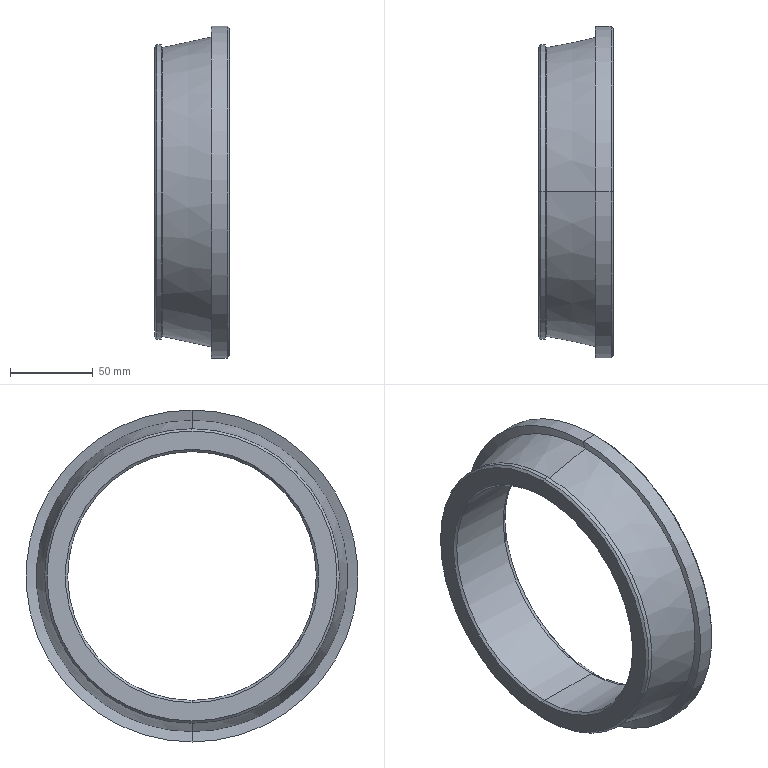Part | SolidWorks | features BaseBody 1 | 1 solid | 22 faces | box 45 x 200.13 x 200.13 mm | volume 409638 mm3 | cone 12 | cylinder 6 | plane 2 | torus 2 | commonest cylinder face diameters 150 x2 177.45 x2 200.13 x2
STEP:
#1=CARTESIAN_POINT('',(4.,0.,-76.333));
#2=VERTEX_POINT('',#1);
#3=CARTESIAN_POINT('',(4.,0.,76.333));
#4=VERTEX_POINT('',#3);
#5=CARTESIAN_POINT('',(4.,0.,0.));
#6=DIRECTION('',(1.,0.,0.));
#7=DIRECTION('',(0.,0.,-1.));
#8=AXIS2_PLACEMENT_3D('',#5,#6,#7);
#9=CIRCLE('',#8,76.333);
#10=EDGE_CURVE('',#2,#4,#9,.T.);
#11=ORIENTED_EDGE('',*,*,#10,.T.);
#12=CARTESIAN_POINT('',(4.,0.,0.));
#13=DIRECTION('',(1.,0.,0.));
#14=DIRECTION('',(0.,0.,-1.));
#15=AXIS2_PLACEMENT_3D('',#12,#13,#14);
#16=CIRCLE('',#15,76.333);
#17=EDGE_CURVE('',#4,#2,#16,.T.);
#18=ORIENTED_EDGE('',*,*,#17,.T.);
#19=EDGE_LOOP('',(#11,#18));
#20=FACE_BOUND('',#19,.T.);
#21=CARTESIAN_POINT('',(4.,0.,87.392));
#22=VERTEX_POINT('',#21);
#23=CARTESIAN_POINT('',(4.,0.,-87.392));
#24=VERTEX_POINT('',#23);
#25=CARTESIAN_POINT('',(4.,0.,0.));
#26=DIRECTION('',(1.,0.,0.));
#27=DIRECTION('',(0.,0.,-1.));
#28=AXIS2_PLACEMENT_3D('',#25,#26,#27);
#29=CIRCLE('',#28,87.392);
#30=EDGE_CURVE('',#22,#24,#29,.T.);
#31=ORIENTED_EDGE('',*,*,#30,.F.);
#32=CARTESIAN_POINT('',(4.,0.,0.));
#33=DIRECTION('',(1.,0.,0.));
#34=DIRECTION('',(0.,0.,-1.));
#35=AXIS2_PLACEMENT_3D('',#32,#33,#34);
#36=CIRCLE('',#35,87.392);
#37=EDGE_CURVE('',#24,#22,#36,.T.);
#38=ORIENTED_EDGE('',*,*,#37,.F.);
#39=EDGE_LOOP('',(#31,#38));
#40=FACE_OUTER_BOUND('',#39,.T.);
#41=CARTESIAN_POINT('',(4.,87.392,0.));
#42=DIRECTION('',(-1.,0.,0.));
#43=DIRECTION('',(0.,0.,1.));
#44=AXIS2_PLACEMENT_3D('',#41,#42,#43);
#45=PLANE('',#44);
#46=ADVANCED_FACE('',(#20,#40),#45,.T.);
#47=CARTESIAN_POINT('',(5.333,0.,88.725));
#48=VERTEX_POINT('',#47);
#49=CARTESIAN_POINT('',(4.,0.,87.392));
#50=DIRECTION('',(0.7071,0.,0.7071));
#51=VECTOR('',#50,1000.);
#52=LINE('',#49,#51);
#53=EDGE_CURVE('',#22,#48,#52,.T.);
#54=ORIENTED_EDGE('',*,*,#53,.T.);
#55=CARTESIAN_POINT('',(5.333,0.,-88.725));
#56=VERTEX_POINT('',#55);
#57=CARTESIAN_POINT('',(5.333,0.,0.));
#58=DIRECTION('',(1.,0.,0.));
#59=DIRECTION('',(0.,0.,-1.));
#60=AXIS2_PLACEMENT_3D('',#57,#58,#59);
#61=CIRCLE('',#60,88.725);
#62=EDGE_CURVE('',#56,#48,#61,.T.);
#63=ORIENTED_EDGE('',*,*,#62,.F.);
#64=CARTESIAN_POINT('',(4.,0.,-87.392));
#65=DIRECTION('',(0.7071,0.,-0.7071));
#66=VECTOR('',#65,1000.);
#67=LINE('',#64,#66);
#68=EDGE_CURVE('',#24,#56,#67,.T.);
#69=ORIENTED_EDGE('',*,*,#68,.F.);
#70=ORIENTED_EDGE('',*,*,#37,.T.);
#71=EDGE_LOOP('',(#54,#63,#69,#70));
#72=FACE_OUTER_BOUND('',#71,.T.);
#73=CARTESIAN_POINT('',(5.333,0.,0.));
#74=DIRECTION('',(1.,0.,0.));
#75=DIRECTION('',(0.,-1.,0.));
#76=AXIS2_PLACEMENT_3D('',#73,#74,#75);
#77=CONICAL_SURFACE('',#76,88.725,0.7854);
#78=ADVANCED_FACE('',(#72),#77,.T.);
#79=ORIENTED_EDGE('',*,*,#53,.F.);
#80=ORIENTED_EDGE('',*,*,#30,.T.);
#81=ORIENTED_EDGE('',*,*,#68,.T.);
#82=CARTESIAN_POINT('',(5.333,0.,0.));
#83=DIRECTION('',(1.,0.,0.));
#84=DIRECTION('',(0.,0.,-1.));
#85=AXIS2_PLACEMENT_3D('',#82,#83,#84);
#86=CIRCLE('',#85,88.725);
#87=EDGE_CURVE('',#48,#56,#86,.T.);
#88=ORIENTED_EDGE('',*,*,#87,.F.);
#89=EDGE_LOOP('',(#79,#80,#81,#88));
#90=FACE_OUTER_BOUND('',#89,.T.);
#91=CARTESIAN_POINT('',(5.333,0.,0.));
#92=DIRECTION('',(1.,0.,0.));
#93=DIRECTION('',(0.,1.,0.));
#94=AXIS2_PLACEMENT_3D('',#91,#92,#93);
#95=CONICAL_SURFACE('',#94,88.725,0.7854);
#96=ADVANCED_FACE('',(#90),#95,.T.);
#97=CARTESIAN_POINT('',(7.994,0.,88.725));
#98=VERTEX_POINT('',#97);
#99=CARTESIAN_POINT('',(5.333,0.,88.725));
#100=DIRECTION('',(1.,0.,0.));
#101=VECTOR('',#100,1000.);
#102=LINE('',#99,#101);
#103=EDGE_CURVE('',#48,#98,#102,.T.);
#104=ORIENTED_EDGE('',*,*,#103,.F.);
#105=ORIENTED_EDGE('',*,*,#87,.T.);
#106=CARTESIAN_POINT('',(7.994,0.,-88.725));
#107=VERTEX_POINT('',#106);
#108=CARTESIAN_POINT('',(5.333,0.,-88.725));
#109=DIRECTION('',(1.,0.,0.));
#110=VECTOR('',#109,1000.);
#111=LINE('',#108,#110);
#112=EDGE_CURVE('',#56,#107,#111,.T.);
#113=ORIENTED_EDGE('',*,*,#112,.T.);
#114=CARTESIAN_POINT('',(7.994,0.,0.));
#115=DIRECTION('',(1.,0.,0.));
#116=DIRECTION('',(0.,0.,-1.));
#117=AXIS2_PLACEMENT_3D('',#114,#115,#116);
#118=CIRCLE('',#117,88.725);
#119=EDGE_CURVE('',#98,#107,#118,.T.);
#120=ORIENTED_EDGE('',*,*,#119,.F.);
#121=EDGE_LOOP('',(#104,#105,#113,#120));
#122=FACE_OUTER_BOUND('',#121,.T.);
#123=CARTESIAN_POINT('',(49.,0.,0.));
#124=DIRECTION('',(1.,0.,0.));
#125=DIRECTION('',(0.,1.,0.));
#126=AXIS2_PLACEMENT_3D('',#123,#124,#125);
#127=CYLINDRICAL_SURFACE('',#126,88.725);
#128=ADVANCED_FACE('',(#122),#127,.T.);
#129=CARTESIAN_POINT('',(8.484,0.,-87.036));
#130=VERTEX_POINT('',#129);
#131=CARTESIAN_POINT('',(8.484,0.,-87.036));
#132=DIRECTION('',(-0.2785,0.,-0.9604));
#133=VECTOR('',#132,1000.);
#134=LINE('',#131,#133);
#135=EDGE_CURVE('',#130,#107,#134,.T.);
#136=ORIENTED_EDGE('',*,*,#135,.F.);
#137=CARTESIAN_POINT('',(8.484,0.,87.036));
#138=VERTEX_POINT('',#137);
#139=CARTESIAN_POINT('',(8.484,0.,0.));
#140=DIRECTION('',(1.,0.,0.));
#141=DIRECTION('',(0.,0.,-1.));
#142=AXIS2_PLACEMENT_3D('',#139,#140,#141);
#143=CIRCLE('',#142,87.036);
#144=EDGE_CURVE('',#138,#130,#143,.T.);
#145=ORIENTED_EDGE('',*,*,#144,.F.);
#146=CARTESIAN_POINT('',(8.484,0.,87.036));
#147=DIRECTION('',(-0.2785,0.,0.9604));
#148=VECTOR('',#147,1000.);
#149=LINE('',#146,#148);
#150=EDGE_CURVE('',#138,#98,#149,.T.);
#151=ORIENTED_EDGE('',*,*,#150,.T.);
#152=ORIENTED_EDGE('',*,*,#119,.T.);
#153=EDGE_LOOP('',(#136,#145,#151,#152));
#154=FACE_OUTER_BOUND('',#153,.T.);
#155=CARTESIAN_POINT('',(8.484,0.,0.));
#156=DIRECTION('',(-1.,0.,0.));
#157=DIRECTION('',(0.,1.,0.));
#158=AXIS2_PLACEMENT_3D('',#155,#156,#157);
#159=CONICAL_SURFACE('',#158,87.036,1.289);
#160=ADVANCED_FACE('',(#154),#159,.T.);
#161=ORIENTED_EDGE('',*,*,#135,.T.);
#162=CARTESIAN_POINT('',(7.994,0.,0.));
#163=DIRECTION('',(1.,0.,0.));
#164=DIRECTION('',(0.,0.,-1.));
#165=AXIS2_PLACEMENT_3D('',#162,#163,#164);
#166=CIRCLE('',#165,88.725);
#167=EDGE_CURVE('',#107,#98,#166,.T.);
#168=ORIENTED_EDGE('',*,*,#167,.T.);
#169=ORIENTED_EDGE('',*,*,#150,.F.);
#170=CARTESIAN_POINT('',(8.484,0.,0.));
#171=DIRECTION('',(1.,0.,0.));
#172=DIRECTION('',(0.,0.,-1.));
#173=AXIS2_PLACEMENT_3D('',#170,#171,#172);
#174=CIRCLE('',#173,87.036);
#175=EDGE_CURVE('',#130,#138,#174,.T.);
#176=ORIENTED_EDGE('',*,*,#175,.F.);
#177=EDGE_LOOP('',(#161,#168,#169,#176));
#178=FACE_OUTER_BOUND('',#177,.T.);
#179=CARTESIAN_POINT('',(8.484,0.,0.));
#180=DIRECTION('',(-1.,0.,0.));
#181=DIRECTION('',(0.,-1.,0.));
#182=AXIS2_PLACEMENT_3D('',#179,#180,#181);
#183=CONICAL_SURFACE('',#182,87.036,1.289);
#184=ADVANCED_FACE('',(#178),#183,.T.);
#185=CARTESIAN_POINT('',(39.843,0.,93.793));
#186=VERTEX_POINT('',#185);
#187=CARTESIAN_POINT('',(8.484,0.,87.036));
#188=DIRECTION('',(0.9776,0.,0.2107));
#189=VECTOR('',#188,1000.);
#190=LINE('',#187,#189);
#191=EDGE_CURVE('',#138,#186,#190,.T.);
#192=ORIENTED_EDGE('',*,*,#191,.T.);
#193=CARTESIAN_POINT('',(39.843,0.,-93.793));
#194=VERTEX_POINT('',#193);
#195=CARTESIAN_POINT('',(39.843,0.,0.));
#196=DIRECTION('',(1.,0.,0.));
#197=DIRECTION('',(0.,0.,-1.));
#198=AXIS2_PLACEMENT_3D('',#195,#196,#197);
#199=CIRCLE('',#198,93.793);
#200=EDGE_CURVE('',#194,#186,#199,.T.);
#201=ORIENTED_EDGE('',*,*,#200,.F.);
#202=CARTESIAN_POINT('',(8.484,0.,-87.036));
#203=DIRECTION('',(0.9776,0.,-0.2107));
#204=VECTOR('',#203,1000.);
#205=LINE('',#202,#204);
#206=EDGE_CURVE('',#130,#194,#205,.T.);
#207=ORIENTED_EDGE('',*,*,#206,.F.);
#208=ORIENTED_EDGE('',*,*,#175,.T.);
#209=EDGE_LOOP('',(#192,#201,#207,#208));
#210=FACE_OUTER_BOUND('',#209,.T.);
#211=CARTESIAN_POINT('',(39.843,0.,0.));
#212=DIRECTION('',(1.,0.,0.));
#213=DIRECTION('',(0.,-1.,0.));
#214=AXIS2_PLACEMENT_3D('',#211,#212,#213);
#215=CONICAL_SURFACE('',#214,93.793,0.2122);
#216=ADVANCED_FACE('',(#210),#215,.T.);
#217=ORIENTED_EDGE('',*,*,#191,.F.);
#218=ORIENTED_EDGE('',*,*,#144,.T.);
#219=ORIENTED_EDGE('',*,*,#206,.T.);
#220=CARTESIAN_POINT('',(39.843,0.,0.));
#221=DIRECTION('',(1.,0.,0.));
#222=DIRECTION('',(0.,0.,-1.));
#223=AXIS2_PLACEMENT_3D('',#220,#221,#222);
#224=CIRCLE('',#223,93.793);
#225=EDGE_CURVE('',#186,#194,#224,.T.);
#226=ORIENTED_EDGE('',*,*,#225,.F.);
#227=EDGE_LOOP('',(#217,#218,#219,#226));
#228=FACE_OUTER_BOUND('',#227,.T.);
#229=CARTESIAN_POINT('',(39.843,0.,0.));
#230=DIRECTION('',(1.,0.,0.));
#231=DIRECTION('',(0.,1.,0.));
#232=AXIS2_PLACEMENT_3D('',#229,#230,#231);
#233=CONICAL_SURFACE('',#232,93.793,0.2122);
#234=ADVANCED_FACE('',(#228),#233,.T.);
#235=CARTESIAN_POINT('',(38.024,0.,-100.065));
#236=VERTEX_POINT('',#235);
#237=CARTESIAN_POINT('',(39.843,0.,-93.793));
#238=DIRECTION('',(-0.2785,0.,-0.9604));
#239=VECTOR('',#238,1000.);
#240=LINE('',#237,#239);
#241=EDGE_CURVE('',#194,#236,#240,.T.);
#242=ORIENTED_EDGE('',*,*,#241,.T.);
#243=CARTESIAN_POINT('',(38.024,0.,100.065));
#244=VERTEX_POINT('',#243);
#245=CARTESIAN_POINT('',(38.024,0.,0.));
#246=DIRECTION('',(1.,0.,0.));
#247=DIRECTION('',(0.,0.,-1.));
#248=AXIS2_PLACEMENT_3D('',#245,#246,#247);
#249=CIRCLE('',#248,100.065);
#250=EDGE_CURVE('',#244,#236,#249,.T.);
#251=ORIENTED_EDGE('',*,*,#250,.F.);
#252=CARTESIAN_POINT('',(39.843,0.,93.793));
#253=DIRECTION('',(-0.2785,0.,0.9604));
#254=VECTOR('',#253,1000.);
#255=LINE('',#252,#254);
#256=EDGE_CURVE('',#186,#244,#255,.T.);
#257=ORIENTED_EDGE('',*,*,#256,.F.);
#258=ORIENTED_EDGE('',*,*,#225,.T.);
#259=EDGE_LOOP('',(#242,#251,#257,#258));
#260=FACE_OUTER_BOUND('',#259,.T.);
#261=CARTESIAN_POINT('',(38.024,0.,0.));
#262=DIRECTION('',(-1.,0.,0.));
#263=DIRECTION('',(0.,1.,0.));
#264=AXIS2_PLACEMENT_3D('',#261,#262,#263);
#265=CONICAL_SURFACE('',#264,100.065,1.289);
#266=ADVANCED_FACE('',(#260),#265,.F.);
#267=ORIENTED_EDGE('',*,*,#241,.F.);
#268=ORIENTED_EDGE('',*,*,#200,.T.);
#269=ORIENTED_EDGE('',*,*,#256,.T.);
#270=CARTESIAN_POINT('',(38.024,0.,0.));
#271=DIRECTION('',(1.,0.,0.));
#272=DIRECTION('',(0.,0.,-1.));
#273=AXIS2_PLACEMENT_3D('',#270,#271,#272);
#274=CIRCLE('',#273,100.065);
#275=EDGE_CURVE('',#236,#244,#274,.T.);
#276=ORIENTED_EDGE('',*,*,#275,.F.);
#277=EDGE_LOOP('',(#267,#268,#269,#276));
#278=FACE_OUTER_BOUND('',#277,.T.);
#279=CARTESIAN_POINT('',(38.024,0.,0.));
#280=DIRECTION('',(-1.,0.,0.));
#281=DIRECTION('',(0.,-1.,0.));
#282=AXIS2_PLACEMENT_3D('',#279,#280,#281);
#283=CONICAL_SURFACE('',#282,100.065,1.289);
#284=ADVANCED_FACE('',(#278),#283,.F.);
#285=CARTESIAN_POINT('',(47.667,0.,100.065));
#286=VERTEX_POINT('',#285);
#287=CARTESIAN_POINT('',(38.024,0.,100.065));
#288=DIRECTION('',(1.,0.,0.));
#289=VECTOR('',#288,1000.);
#290=LINE('',#287,#289);
#291=EDGE_CURVE('',#244,#286,#290,.T.);
#292=ORIENTED_EDGE('',*,*,#291,.T.);
#293=CARTESIAN_POINT('',(47.667,0.,-100.065));
#294=VERTEX_POINT('',#293);
#295=CARTESIAN_POINT('',(47.667,0.,0.));
#296=DIRECTION('',(1.,0.,0.));
#297=DIRECTION('',(0.,0.,-1.));
#298=AXIS2_PLACEMENT_3D('',#295,#296,#297);
#299=CIRCLE('',#298,100.065);
#300=EDGE_CURVE('',#294,#286,#299,.T.);
#301=ORIENTED_EDGE('',*,*,#300,.F.);
#302=CARTESIAN_POINT('',(38.024,0.,-100.065));
#303=DIRECTION('',(1.,0.,0.));
#304=VECTOR('',#303,1000.);
#305=LINE('',#302,#304);
#306=EDGE_CURVE('',#236,#294,#305,.T.);
#307=ORIENTED_EDGE('',*,*,#306,.F.);
#308=ORIENTED_EDGE('',*,*,#275,.T.);
#309=EDGE_LOOP('',(#292,#301,#307,#308));
#310=FACE_OUTER_BOUND('',#309,.T.);
#311=CARTESIAN_POINT('',(49.,0.,0.));
#312=DIRECTION('',(1.,0.,0.));
#313=DIRECTION('',(0.,-1.,0.));
#314=AXIS2_PLACEMENT_3D('',#311,#312,#313);
#315=CYLINDRICAL_SURFACE('',#314,100.065);
#316=ADVANCED_FACE('',(#310),#315,.T.);
#317=ORIENTED_EDGE('',*,*,#291,.F.);
#318=ORIENTED_EDGE('',*,*,#250,.T.);
#319=ORIENTED_EDGE('',*,*,#306,.T.);
#320=CARTESIAN_POINT('',(47.667,0.,0.));
#321=DIRECTION('',(1.,0.,0.));
#322=DIRECTION('',(0.,0.,-1.));
#323=AXIS2_PLACEMENT_3D('',#320,#321,#322);
#324=CIRCLE('',#323,100.065);
#325=EDGE_CURVE('',#286,#294,#324,.T.);
#326=ORIENTED_EDGE('',*,*,#325,.F.);
#327=EDGE_LOOP('',(#317,#318,#319,#326));
#328=FACE_OUTER_BOUND('',#327,.T.);
#329=CARTESIAN_POINT('',(49.,0.,0.));
#330=DIRECTION('',(1.,0.,0.));
#331=DIRECTION('',(0.,1.,0.));
#332=AXIS2_PLACEMENT_3D('',#329,#330,#331);
#333=CYLINDRICAL_SURFACE('',#332,100.065);
#334=ADVANCED_FACE('',(#328),#333,.T.);
#335=CARTESIAN_POINT('',(49.,0.,-98.732));
#336=VERTEX_POINT('',#335);
#337=CARTESIAN_POINT('',(49.,0.,-98.732));
#338=DIRECTION('',(-0.7071,0.,-0.7071));
#339=VECTOR('',#338,1000.);
#340=LINE('',#337,#339);
#341=EDGE_CURVE('',#336,#294,#340,.T.);
#342=ORIENTED_EDGE('',*,*,#341,.F.);
#343=CARTESIAN_POINT('',(49.,0.,98.732));
#344=VERTEX_POINT('',#343);
#345=CARTESIAN_POINT('',(49.,0.,0.));
#346=DIRECTION('',(1.,0.,0.));
#347=DIRECTION('',(0.,0.,-1.));
#348=AXIS2_PLACEMENT_3D('',#345,#346,#347);
#349=CIRCLE('',#348,98.732);
#350=EDGE_CURVE('',#344,#336,#349,.T.);
#351=ORIENTED_EDGE('',*,*,#350,.F.);
#352=CARTESIAN_POINT('',(49.,0.,98.732));
#353=DIRECTION('',(-0.7071,0.,0.7071));
#354=VECTOR('',#353,1000.);
#355=LINE('',#352,#354);
#356=EDGE_CURVE('',#344,#286,#355,.T.);
#357=ORIENTED_EDGE('',*,*,#356,.T.);
#358=ORIENTED_EDGE('',*,*,#325,.T.);
#359=EDGE_LOOP('',(#342,#351,#357,#358));
#360=FACE_OUTER_BOUND('',#359,.T.);
#361=CARTESIAN_POINT('',(49.,0.,0.));
#362=DIRECTION('',(-1.,0.,0.));
#363=DIRECTION('',(0.,1.,0.));
#364=AXIS2_PLACEMENT_3D('',#361,#362,#363);
#365=CONICAL_SURFACE('',#364,98.732,0.7854);
#366=ADVANCED_FACE('',(#360),#365,.T.);
#367=ORIENTED_EDGE('',*,*,#341,.T.);
#368=ORIENTED_EDGE('',*,*,#300,.T.);
#369=ORIENTED_EDGE('',*,*,#356,.F.);
#370=CARTESIAN_POINT('',(49.,0.,0.));
#371=DIRECTION('',(1.,0.,0.));
#372=DIRECTION('',(0.,0.,-1.));
#373=AXIS2_PLACEMENT_3D('',#370,#371,#372);
#374=CIRCLE('',#373,98.732);
#375=EDGE_CURVE('',#336,#344,#374,.T.);
#376=ORIENTED_EDGE('',*,*,#375,.F.);
#377=EDGE_LOOP('',(#367,#368,#369,#376));
#378=FACE_OUTER_BOUND('',#377,.T.);
#379=CARTESIAN_POINT('',(49.,0.,0.));
#380=DIRECTION('',(-1.,0.,0.));
#381=DIRECTION('',(0.,-1.,0.));
#382=AXIS2_PLACEMENT_3D('',#379,#380,#381);
#383=CONICAL_SURFACE('',#382,98.732,0.7854);
#384=ADVANCED_FACE('',(#378),#383,.T.);
#385=ORIENTED_EDGE('',*,*,#375,.T.);
#386=ORIENTED_EDGE('',*,*,#350,.T.);
#387=EDGE_LOOP('',(#385,#386));
#388=FACE_OUTER_BOUND('',#387,.T.);
#389=CARTESIAN_POINT('',(49.,-75.133,-24.412));
#390=VERTEX_POINT('',#389);
#391=CARTESIAN_POINT('',(49.,75.133,24.412));
#392=VERTEX_POINT('',#391);
#393=CARTESIAN_POINT('',(49.,-75.133,-24.412));
#394=CARTESIAN_POINT('',(49.,-73.536,-29.33));
#395=CARTESIAN_POINT('',(49.,-71.454,-34.09));
#396=CARTESIAN_POINT('',(49.,-66.401,-43.112));
#397=CARTESIAN_POINT('',(49.,-63.43,-47.375));
#398=CARTESIAN_POINT('',(49.,-56.714,-55.238));
#399=CARTESIAN_POINT('',(49.,-52.969,-58.839));
#400=CARTESIAN_POINT('',(49.,-44.848,-65.241));
#401=CARTESIAN_POINT('',(49.,-40.472,-68.042));
#402=CARTESIAN_POINT('',(49.,-31.258,-72.737));
#403=CARTESIAN_POINT('',(49.,-26.42,-74.63));
#404=CARTESIAN_POINT('',(49.,-16.467,-77.437));
#405=CARTESIAN_POINT('',(49.,-11.353,-78.351));
#406=CARTESIAN_POINT('',(49.,-1.044,-79.162));
#407=CARTESIAN_POINT('',(49.,4.151,-79.06));
#408=CARTESIAN_POINT('',(49.,14.42,-77.845));
#409=CARTESIAN_POINT('',(49.,19.495,-76.731));
#410=CARTESIAN_POINT('',(49.,29.33,-73.536));
#411=CARTESIAN_POINT('',(49.,34.09,-71.454));
#412=CARTESIAN_POINT('',(49.,43.112,-66.401));
#413=CARTESIAN_POINT('',(49.,47.375,-63.43));
#414=CARTESIAN_POINT('',(49.,55.238,-56.714));
#415=CARTESIAN_POINT('',(49.,58.839,-52.969));
#416=CARTESIAN_POINT('',(49.,65.241,-44.848));
#417=CARTESIAN_POINT('',(49.,68.042,-40.472));
#418=CARTESIAN_POINT('',(49.,72.737,-31.258));
#419=CARTESIAN_POINT('',(49.,74.63,-26.42));
#420=CARTESIAN_POINT('',(49.,77.437,-16.467));
#421=CARTESIAN_POINT('',(49.,78.351,-11.353));
#422=CARTESIAN_POINT('',(49.,79.162,-1.044));
#423=CARTESIAN_POINT('',(49.,79.06,4.151));
#424=CARTESIAN_POINT('',(49.,77.845,14.42));
#425=CARTESIAN_POINT('',(49.,76.731,19.495));
#426=CARTESIAN_POINT('',(49.,75.133,24.412));
#427=B_SPLINE_CURVE_WITH_KNOTS('',3,(#393,#394,#395,#396,#397,#398,#399,#400,#401,#402,#403,#404,#405,#406,#407,#408,#409,#410,#411,#412,#413,#414,#415,#416,#417,#418,#419,#420,#421,#422,#423,#424,#425,#426),.UNSPECIFIED.,.F.,.F.,(4,2,2,2,2,2,2,2,2,2,2,2,2,2,2,2,4),(0.,0.1963,0.3927,0.589,0.7854,0.9817,1.178,1.374,1.571,1.767,1.963,2.16,2.356,2.553,2.749,2.945,3.142),.UNSPECIFIED.);
#428=EDGE_CURVE('',#390,#392,#427,.T.);
#429=ORIENTED_EDGE('',*,*,#428,.F.);
#430=CARTESIAN_POINT('',(49.,75.133,24.412));
#431=CARTESIAN_POINT('',(49.,73.536,29.33));
#432=CARTESIAN_POINT('',(49.,71.454,34.09));
#433=CARTESIAN_POINT('',(49.,66.401,43.112));
#434=CARTESIAN_POINT('',(49.,63.43,47.375));
#435=CARTESIAN_POINT('',(49.,56.714,55.238));
#436=CARTESIAN_POINT('',(49.,52.969,58.839));
#437=CARTESIAN_POINT('',(49.,44.848,65.241));
#438=CARTESIAN_POINT('',(49.,40.472,68.042));
#439=CARTESIAN_POINT('',(49.,31.258,72.737));
#440=CARTESIAN_POINT('',(49.,26.42,74.63));
#441=CARTESIAN_POINT('',(49.,16.467,77.437));
#442=CARTESIAN_POINT('',(49.,11.353,78.351));
#443=CARTESIAN_POINT('',(49.,1.044,79.162));
#444=CARTESIAN_POINT('',(49.,-4.151,79.06));
#445=CARTESIAN_POINT('',(49.,-14.42,77.845));
#446=CARTESIAN_POINT('',(49.,-19.495,76.731));
#447=CARTESIAN_POINT('',(49.,-29.33,73.536));
#448=CARTESIAN_POINT('',(49.,-34.09,71.454));
#449=CARTESIAN_POINT('',(49.,-43.112,66.401));
#450=CARTESIAN_POINT('',(49.,-47.375,63.43));
#451=CARTESIAN_POINT('',(49.,-55.238,56.714));
#452=CARTESIAN_POINT('',(49.,-58.839,52.969));
#453=CARTESIAN_POINT('',(49.,-65.241,44.848));
#454=CARTESIAN_POINT('',(49.,-68.042,40.472));
#455=CARTESIAN_POINT('',(49.,-72.737,31.258));
#456=CARTESIAN_POINT('',(49.,-74.63,26.42));
#457=CARTESIAN_POINT('',(49.,-77.437,16.467));
#458=CARTESIAN_POINT('',(49.,-78.351,11.353));
#459=CARTESIAN_POINT('',(49.,-79.162,1.044));
#460=CARTESIAN_POINT('',(49.,-79.06,-4.151));
#461=CARTESIAN_POINT('',(49.,-77.845,-14.42));
#462=CARTESIAN_POINT('',(49.,-76.731,-19.495));
#463=CARTESIAN_POINT('',(49.,-75.133,-24.412));
#464=B_SPLINE_CURVE_WITH_KNOTS('',3,(#430,#431,#432,#433,#434,#435,#436,#437,#438,#439,#440,#441,#442,#443,#444,#445,#446,#447,#448,#449,#450,#451,#452,#453,#454,#455,#456,#457,#458,#459,#460,#461,#462,#463),.UNSPECIFIED.,.F.,.F.,(4,2,2,2,2,2,2,2,2,2,2,2,2,2,2,2,4),(0.,0.1963,0.3927,0.589,0.7854,0.9817,1.178,1.374,1.571,1.767,1.963,2.16,2.356,2.553,2.749,2.945,3.142),.UNSPECIFIED.);
#465=EDGE_CURVE('',#392,#390,#464,.T.);
#466=ORIENTED_EDGE('',*,*,#465,.F.);
#467=EDGE_LOOP('',(#429,#466));
#468=FACE_BOUND('',#467,.T.);
#469=CARTESIAN_POINT('',(49.,79.,0.));
#470=DIRECTION('',(1.,0.,0.));
#471=DIRECTION('',(0.,0.,-1.));
#472=AXIS2_PLACEMENT_3D('',#469,#470,#471);
#473=PLANE('',#472);
#474=ADVANCED_FACE('',(#388,#468),#473,.T.);
#475=CARTESIAN_POINT('',(45.,-71.329,-23.176));
#476=VERTEX_POINT('',#475);
#477=CARTESIAN_POINT('',(45.,-75.133,-24.412));
#478=DIRECTION('',(0.,0.309,-0.9511));
#479=DIRECTION('',(0.,0.9511,0.309));
#480=AXIS2_PLACEMENT_3D('',#477,#478,#479);
#481=CIRCLE('',#480,4.);
#482=EDGE_CURVE('',#476,#390,#481,.T.);
#483=ORIENTED_EDGE('',*,*,#482,.F.);
#484=CARTESIAN_POINT('',(45.,0.,75.));
#485=VERTEX_POINT('',#484);
#486=CARTESIAN_POINT('',(45.,0.,0.));
#487=DIRECTION('',(1.,0.,0.));
#488=DIRECTION('',(0.,0.,-1.));
#489=AXIS2_PLACEMENT_3D('',#486,#487,#488);
#490=CIRCLE('',#489,75.);
#491=EDGE_CURVE('',#485,#476,#490,.T.);
#492=ORIENTED_EDGE('',*,*,#491,.F.);
#493=CARTESIAN_POINT('',(45.,71.329,23.176));
#494=VERTEX_POINT('',#493);
#495=CARTESIAN_POINT('',(45.,0.,0.));
#496=DIRECTION('',(1.,0.,0.));
#497=DIRECTION('',(0.,0.,-1.));
#498=AXIS2_PLACEMENT_3D('',#495,#496,#497);
#499=CIRCLE('',#498,75.);
#500=EDGE_CURVE('',#494,#485,#499,.T.);
#501=ORIENTED_EDGE('',*,*,#500,.F.);
#502=CARTESIAN_POINT('',(45.,75.133,24.412));
#503=DIRECTION('',(0.,-0.309,0.9511));
#504=DIRECTION('',(0.,-0.9511,-0.309));
#505=AXIS2_PLACEMENT_3D('',#502,#503,#504);
#506=CIRCLE('',#505,4.);
#507=EDGE_CURVE('',#494,#392,#506,.T.);
#508=ORIENTED_EDGE('',*,*,#507,.T.);
#509=ORIENTED_EDGE('',*,*,#465,.T.);
#510=EDGE_LOOP('',(#483,#492,#501,#508,#509));
#511=FACE_OUTER_BOUND('',#510,.T.);
#512=CARTESIAN_POINT('',(45.,0.,0.));
#513=DIRECTION('',(1.,0.,0.));
#514=DIRECTION('',(0.,0.309,-0.9511));
#515=AXIS2_PLACEMENT_3D('',#512,#513,#514);
#516=TOROIDAL_SURFACE('',#515,79.,4.);
#517=ADVANCED_FACE('',(#511),#516,.T.);
#518=ORIENTED_EDGE('',*,*,#482,.T.);
#519=ORIENTED_EDGE('',*,*,#428,.T.);
#520=ORIENTED_EDGE('',*,*,#507,.F.);
#521=CARTESIAN_POINT('',(45.,0.,-75.));
#522=VERTEX_POINT('',#521);
#523=CARTESIAN_POINT('',(45.,0.,0.));
#524=DIRECTION('',(1.,0.,0.));
#525=DIRECTION('',(0.,0.,-1.));
#526=AXIS2_PLACEMENT_3D('',#523,#524,#525);
#527=CIRCLE('',#526,75.);
#528=EDGE_CURVE('',#522,#494,#527,.T.);
#529=ORIENTED_EDGE('',*,*,#528,.F.);
#530=CARTESIAN_POINT('',(45.,0.,0.));
#531=DIRECTION('',(1.,0.,0.));
#532=DIRECTION('',(0.,0.,-1.));
#533=AXIS2_PLACEMENT_3D('',#530,#531,#532);
#534=CIRCLE('',#533,75.);
#535=EDGE_CURVE('',#476,#522,#534,.T.);
#536=ORIENTED_EDGE('',*,*,#535,.F.);
#537=EDGE_LOOP('',(#518,#519,#520,#529,#536));
#538=FACE_OUTER_BOUND('',#537,.T.);
#539=CARTESIAN_POINT('',(45.,0.,0.));
#540=DIRECTION('',(1.,0.,0.));
#541=DIRECTION('',(0.,-0.309,0.9511));
#542=AXIS2_PLACEMENT_3D('',#539,#540,#541);
#543=TOROIDAL_SURFACE('',#542,79.,4.);
#544=ADVANCED_FACE('',(#538),#543,.T.);
#545=CARTESIAN_POINT('',(5.333,0.,75.));
#546=VERTEX_POINT('',#545);
#547=CARTESIAN_POINT('',(5.333,0.,75.));
#548=DIRECTION('',(1.,0.,0.));
#549=VECTOR('',#548,1000.);
#550=LINE('',#547,#549);
#551=EDGE_CURVE('',#546,#485,#550,.T.);
#552=ORIENTED_EDGE('',*,*,#551,.T.);
#553=ORIENTED_EDGE('',*,*,#491,.T.);
#554=ORIENTED_EDGE('',*,*,#535,.T.);
#555=CARTESIAN_POINT('',(5.333,0.,-75.));
#556=VERTEX_POINT('',#555);
#557=CARTESIAN_POINT('',(5.333,0.,-75.));
#558=DIRECTION('',(1.,0.,0.));
#559=VECTOR('',#558,1000.);
#560=LINE('',#557,#559);
#561=EDGE_CURVE('',#556,#522,#560,.T.);
#562=ORIENTED_EDGE('',*,*,#561,.F.);
#563=CARTESIAN_POINT('',(5.333,0.,0.));
#564=DIRECTION('',(1.,0.,0.));
#565=DIRECTION('',(0.,0.,-1.));
#566=AXIS2_PLACEMENT_3D('',#563,#564,#565);
#567=CIRCLE('',#566,75.);
#568=EDGE_CURVE('',#546,#556,#567,.T.);
#569=ORIENTED_EDGE('',*,*,#568,.F.);
#570=EDGE_LOOP('',(#552,#553,#554,#562,#569));
#571=FACE_OUTER_BOUND('',#570,.T.);
#572=CARTESIAN_POINT('',(49.,0.,0.));
#573=DIRECTION('',(1.,0.,0.));
#574=DIRECTION('',(0.,1.,0.));
#575=AXIS2_PLACEMENT_3D('',#572,#573,#574);
#576=CYLINDRICAL_SURFACE('',#575,75.);
#577=ADVANCED_FACE('',(#571),#576,.F.);
#578=CARTESIAN_POINT('',(5.333,0.,-75.));
#579=DIRECTION('',(-0.7071,0.,-0.7071));
#580=VECTOR('',#579,1000.);
#581=LINE('',#578,#580);
#582=EDGE_CURVE('',#556,#2,#581,.T.);
#583=ORIENTED_EDGE('',*,*,#582,.T.);
#584=ORIENTED_EDGE('',*,*,#17,.F.);
#585=CARTESIAN_POINT('',(5.333,0.,75.));
#586=DIRECTION('',(-0.7071,0.,0.7071));
#587=VECTOR('',#586,1000.);
#588=LINE('',#585,#587);
#589=EDGE_CURVE('',#546,#4,#588,.T.);
#590=ORIENTED_EDGE('',*,*,#589,.F.);
#591=ORIENTED_EDGE('',*,*,#568,.T.);
#592=EDGE_LOOP('',(#583,#584,#590,#591));
#593=FACE_OUTER_BOUND('',#592,.T.);
#594=CARTESIAN_POINT('',(4.,0.,0.));
#595=DIRECTION('',(-1.,0.,0.));
#596=DIRECTION('',(0.,1.,0.));
#597=AXIS2_PLACEMENT_3D('',#594,#595,#596);
#598=CONICAL_SURFACE('',#597,76.333,0.7854);
#599=ADVANCED_FACE('',(#593),#598,.F.);
#600=ORIENTED_EDGE('',*,*,#582,.F.);
#601=CARTESIAN_POINT('',(5.333,0.,0.));
#602=DIRECTION('',(1.,0.,0.));
#603=DIRECTION('',(0.,0.,-1.));
#604=AXIS2_PLACEMENT_3D('',#601,#602,#603);
#605=CIRCLE('',#604,75.);
#606=EDGE_CURVE('',#556,#546,#605,.T.);
#607=ORIENTED_EDGE('',*,*,#606,.T.);
#608=ORIENTED_EDGE('',*,*,#589,.T.);
#609=ORIENTED_EDGE('',*,*,#10,.F.);
#610=EDGE_LOOP('',(#600,#607,#608,#609));
#611=FACE_OUTER_BOUND('',#610,.T.);
#612=CARTESIAN_POINT('',(4.,0.,0.));
#613=DIRECTION('',(-1.,0.,0.));
#614=DIRECTION('',(0.,-1.,0.));
#615=AXIS2_PLACEMENT_3D('',#612,#613,#614);
#616=CONICAL_SURFACE('',#615,76.333,0.7854);
#617=ADVANCED_FACE('',(#611),#616,.F.);
#618=ORIENTED_EDGE('',*,*,#551,.F.);
#619=ORIENTED_EDGE('',*,*,#606,.F.);
#620=ORIENTED_EDGE('',*,*,#561,.T.);
#621=ORIENTED_EDGE('',*,*,#528,.T.);
#622=ORIENTED_EDGE('',*,*,#500,.T.);
#623=EDGE_LOOP('',(#618,#619,#620,#621,#622));
#624=FACE_OUTER_BOUND('',#623,.T.);
#625=CARTESIAN_POINT('',(49.,0.,0.));
#626=DIRECTION('',(1.,0.,0.));
#627=DIRECTION('',(0.,-1.,0.));
#628=AXIS2_PLACEMENT_3D('',#625,#626,#627);
#629=CYLINDRICAL_SURFACE('',#628,75.);
#630=ADVANCED_FACE('',(#624),#629,.F.);
#631=ORIENTED_EDGE('',*,*,#103,.T.);
#632=ORIENTED_EDGE('',*,*,#167,.F.);
#633=ORIENTED_EDGE('',*,*,#112,.F.);
#634=ORIENTED_EDGE('',*,*,#62,.T.);
#635=EDGE_LOOP('',(#631,#632,#633,#634));
#636=FACE_OUTER_BOUND('',#635,.T.);
#637=CARTESIAN_POINT('',(49.,0.,0.));
#638=DIRECTION('',(1.,0.,0.));
#639=DIRECTION('',(0.,-1.,0.));
#640=AXIS2_PLACEMENT_3D('',#637,#638,#639);
#641=CYLINDRICAL_SURFACE('',#640,88.725);
#642=ADVANCED_FACE('',(#636),#641,.T.);
#643=CLOSED_SHELL('',(#46,#78,#96,#128,#160,#184,#216,#234,#266,#284,#316,#334,#366,#384,#474,#517,#544,#577,#599,#617,#630,#642));
#644=MANIFOLD_SOLID_BREP('',#643);
#645=CARTESIAN_POINT('',(0.,0.,0.));
#646=DIRECTION('',(0.,0.,1.));
#647=DIRECTION('',(1.,0.,0.));
#648=AXIS2_PLACEMENT_3D('',#645,#646,#647);
#649=(LENGTH_UNIT()NAMED_UNIT(*)SI_UNIT(.MILLI.,.METRE.));
#650=UNCERTAINTY_MEASURE_WITH_UNIT(LENGTH_MEASURE(0.00001),#649,'','');
#651=(NAMED_UNIT(*)PLANE_ANGLE_UNIT()SI_UNIT($,.RADIAN.));
#652=(NAMED_UNIT(*)SI_UNIT($,.STERADIAN.)SOLID_ANGLE_UNIT());
#653=(GEOMETRIC_REPRESENTATION_CONTEXT(3)GLOBAL_UNCERTAINTY_ASSIGNED_CONTEXT((#650))GLOBAL_UNIT_ASSIGNED_CONTEXT((#649,#651,#652))REPRESENTATION_CONTEXT('',''));
#654=ADVANCED_BREP_SHAPE_REPRESENTATION('',(#644,#648),#653);